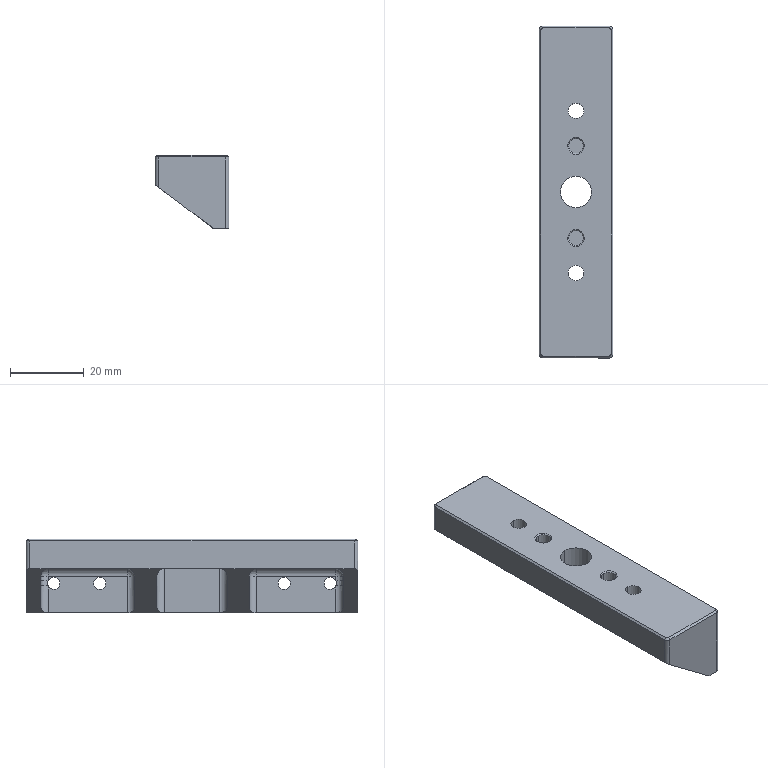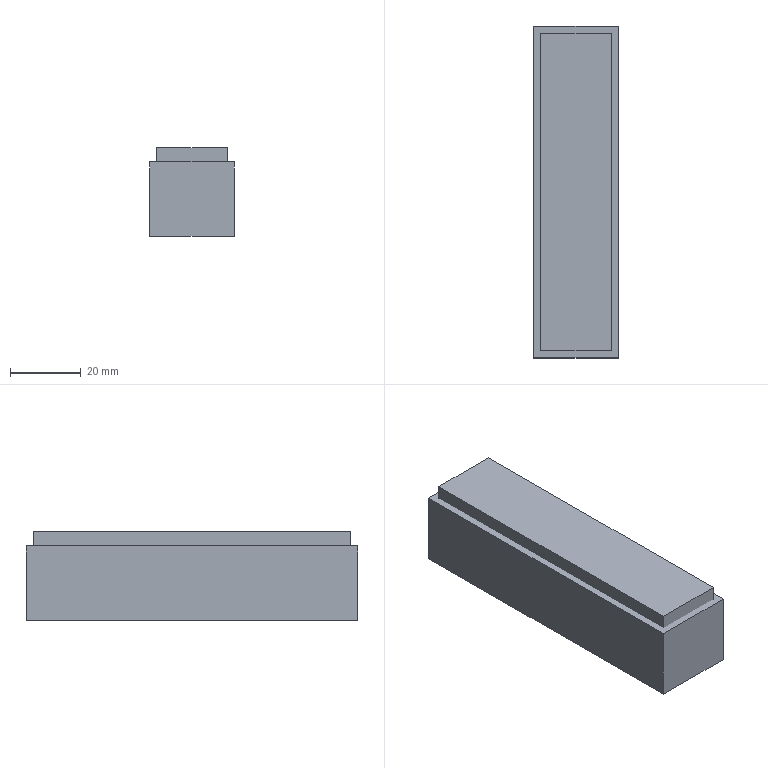CAM job | NX | 3+2 milling, drilling | part box 20 x 90 x 20 mm | stock box 24 x 94 x 25 mm
Tools:
number,name,description,diameter,corner_radius,flute_length,length,flutes
19,D80,Milling Tool-5 Parameters,80.0,0.0,50.0,75.0,2
1,D6A45,Milling Tool-5 Parameters,6.0,0.0,50.0,75.0,2
4,4.2ZT,Drilling Tool,4.2,0.0,35.0,50.0,2
18,3.8ZT,Drilling Tool,3.8,0.0,35.0,50.0,2
16,8.5ZT,Drilling Tool,8.5,0.0,35.0,50.0,2
17,D3,Milling Tool-5 Parameters,3.0,0.0,50.0,75.0,2
15,D10,Milling Tool-5 Parameters,10.0,0.0,50.0,75.0,2
14,D10JING,Milling Tool-5 Parameters,10.0,0.0,50.0,75.0,2
24,D4R0.5,Milling Tool-5 Parameters,4.0,0.5,50.0,75.0,2
3,3.3ZT,Drilling Tool,3.3,0.0,35.0,50.0,2
Operations:
program,operation,operation_type,tool,method,geometry_group,spindle_rpm,surface_speed,feed_per_tooth,feed_cut,feed_plunge,cut_length_mm,path_length_mm,cut_time_min,machine_time_min
1,FLOOR_WALL,VolumeBased25DMillingOperation,D80,METHOD,A,6500.0,1633.0,0.1154,1500.0,100.0,186.0,240.0,0.124,0.1294
1,DRILLING,Operation,D6A45,METHOD,A,5000.0,94.0,0.035,350.0,0.0,20.0,157.635,0.0571,0.0709
1,DRILLING_COPY_COPY,Operation,4.2ZT,METHOD,A,2000.0,26.0,0.075,300.0,0.0,27.524,162.149,0.0917,0.1052
1,DRILLING_COPY_COPY_1_COPY,Operation,3.8ZT,METHOD,A,2000.0,20.0,0.05,200.0,0.0,20.283,128.746,0.1014,0.1123
1,DRILLING_COPY_COPY_COPY,Operation,8.5ZT,METHOD,A,2000.0,26.0,0.075,300.0,0.0,15.054,90.107,0.0502,0.0577
1,ZLEVEL_PROFILE,ZLevelMilling,D10,METHOD,A,9500.0,298.0,0.1579,3000.0,1000.0,5305.89,5382.89,1.8,1.808
1,ZLEVEL_PROFILE_COPY_1,ZLevelMilling,D10JING,METHOD,A,9500.0,298.0,0.0632,1200.0,1000.0,662.006,739.006,0.6201,0.6278
1,PLANAR_MILL_COPY_COPY_COPY,PlanarMilling,D6A45,METHOD,A,9500.0,179.0,0.0658,1250.0,100.0,91.543,432.308,0.0732,0.1073
1,PLANAR_MILL_COPY_COPY_COPY_COPY,PlanarMilling,D6A45,METHOD,A,9500.0,179.0,0.0658,1250.0,100.0,228.136,287.136,0.1825,0.1884
1,刀补,CylinderMilling,D3,METHOD,A,9500.0,89.0,0.0658,1250.0,100.0,47.44,203.44,0.038,0.0536
2,FLOOR_WALL_COPY,VolumeBased25DMillingOperation,D80,METHOD,B,6500.0,1633.0,0.1154,1500.0,100.0,910.0,1864.001,0.6067,0.7021
2,CAVITY_MILL,CavityMilling,D10,METHOD,B,9500.0,298.0,0.1842,3500.0,1000.0,4233.022,4632.137,1.342,1.382
2,FIXED_CONTOUR,SurfaceContour,D4R0.5,METHOD,B,9500.0,119.0,0.1579,3000.0,100.0,24690.653,26310.257,8.23,8.392
2,PLANAR_MILL_COPY_COPY_COPY_COPY_1,PlanarMilling,D6A45,METHOD,B,9500.0,179.0,0.0658,1250.0,100.0,106.68,165.68,0.0853,0.0912
3,DRILLING_COPY,Operation,D6A45,METHOD,C,5000.0,94.0,0.035,350.0,0.0,24.0,199.599,0.0686,0.0861
3,DRILLING_COPY_1,Operation,3.3ZT,METHOD,C,2000.0,20.0,0.05,200.0,0.0,37.966,220.731,0.1898,0.2081
3,DRILLING_COPY_COPY_1_COPY_COPY,Operation,3.8ZT,METHOD,C,2000.0,20.0,0.05,200.0,0.0,16.283,120.746,0.0814,0.0919
3,PLANAR_MILL_COPY_COPY_COPY_COPY_2,PlanarMilling,D6A45,METHOD,C,9500.0,179.0,0.0658,1250.0,100.0,82.104,514.784,0.0657,0.109
3,刀补_COPY,CylinderMilling,D3,METHOD,C,9500.0,89.0,0.0658,1250.0,100.0,35.444,187.444,0.0284,0.0436